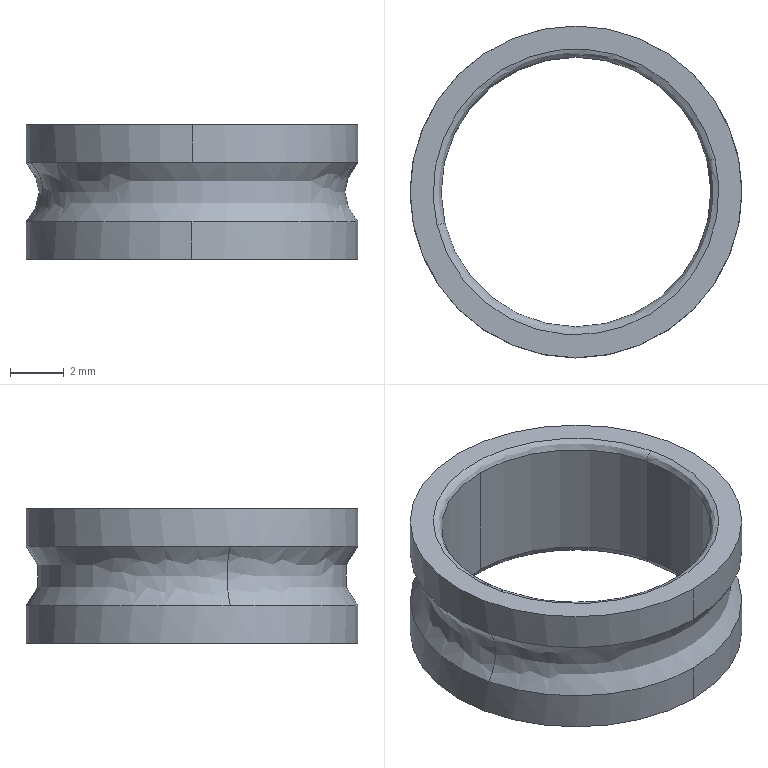Part | SolidWorks | features BaseBody 1 | 1 solid | 14 faces | box 12.3 x 12.3 x 5 mm | volume 173.294 mm3 | spline 6 | cylinder 6 | plane 2 | commonest cylinder face diameters 12.3 x4 10 x2
STEP:
#1=CARTESIAN_POINT('',(465.27,-93.215,300.844));
#2=VERTEX_POINT('',#1);
#3=CARTESIAN_POINT('',(460.405,-99.367,300.844));
#4=VERTEX_POINT('',#3);
#5=CARTESIAN_POINT('',(465.27,-98.215,300.844));
#6=DIRECTION('',(0.000000004,-0.00000001,1.));
#7=DIRECTION('',(0.,1.,0.00000001));
#8=AXIS2_PLACEMENT_3D('',#5,#6,#7);
#9=CIRCLE('',#8,5.);
#10=EDGE_CURVE('',#2,#4,#9,.T.);
#11=ORIENTED_EDGE('',*,*,#10,.T.);
#12=CARTESIAN_POINT('',(460.113,-99.436,300.544));
#13=VERTEX_POINT('',#12);
#14=CARTESIAN_POINT('',(460.113,-99.436,300.844));
#15=DIRECTION('',(-0.2304,0.9731,0.00000001));
#16=DIRECTION('',(-0.9731,-0.2304,0.000000002));
#17=AXIS2_PLACEMENT_3D('',#14,#15,#16);
#18=CIRCLE('',#17,0.3);
#19=EDGE_CURVE('',#4,#13,#18,.T.);
#20=ORIENTED_EDGE('',*,*,#19,.T.);
#21=CARTESIAN_POINT('',(470.428,-96.994,300.544));
#22=VERTEX_POINT('',#21);
#23=CARTESIAN_POINT('',(460.113,-99.436,300.544));
#24=CARTESIAN_POINT('',(457.671,-89.121,300.544));
#25=CARTESIAN_POINT('',(467.985,-86.679,300.544));
#26=CARTESIAN_POINT('',(470.428,-96.994,300.544));
#27=(BOUNDED_CURVE()B_SPLINE_CURVE(3,(#23,#24,#25,#26),.UNSPECIFIED.,.F.,.F.)B_SPLINE_CURVE_WITH_KNOTS((4,4),(0.,1.),.UNSPECIFIED.)CURVE()GEOMETRIC_REPRESENTATION_ITEM()RATIONAL_B_SPLINE_CURVE((1.,0.3333,0.3333,1.))REPRESENTATION_ITEM(''));
#28=EDGE_CURVE('',#13,#22,#27,.T.);
#29=ORIENTED_EDGE('',*,*,#28,.T.);
#30=CARTESIAN_POINT('',(470.136,-97.063,300.844));
#31=VERTEX_POINT('',#30);
#32=CARTESIAN_POINT('',(470.428,-96.994,300.844));
#33=DIRECTION('',(0.2304,-0.9731,-0.00000001));
#34=DIRECTION('',(0.9731,0.2304,-0.000000002));
#35=AXIS2_PLACEMENT_3D('',#32,#33,#34);
#36=CIRCLE('',#35,0.3);
#37=EDGE_CURVE('',#31,#22,#36,.T.);
#38=ORIENTED_EDGE('',*,*,#37,.F.);
#39=CARTESIAN_POINT('',(465.27,-98.215,300.844));
#40=DIRECTION('',(0.000000004,-0.00000001,1.));
#41=DIRECTION('',(0.,1.,0.00000001));
#42=AXIS2_PLACEMENT_3D('',#39,#40,#41);
#43=CIRCLE('',#42,5.);
#44=EDGE_CURVE('',#31,#2,#43,.T.);
#45=ORIENTED_EDGE('',*,*,#44,.T.);
#46=EDGE_LOOP('',(#11,#20,#29,#38,#45));
#47=FACE_OUTER_BOUND('',#46,.T.);
#48=CARTESIAN_POINT('',(460.405,-99.367,300.844));
#49=CARTESIAN_POINT('',(458.101,-89.636,300.844));
#50=CARTESIAN_POINT('',(467.832,-87.332,300.844));
#51=CARTESIAN_POINT('',(470.136,-97.063,300.844));
#52=CARTESIAN_POINT('',(460.405,-99.367,300.669));
#53=CARTESIAN_POINT('',(458.101,-89.636,300.669));
#54=CARTESIAN_POINT('',(467.832,-87.332,300.669));
#55=CARTESIAN_POINT('',(470.136,-97.063,300.669));
#56=CARTESIAN_POINT('',(460.284,-99.396,300.544));
#57=CARTESIAN_POINT('',(457.923,-89.423,300.544));
#58=CARTESIAN_POINT('',(467.895,-87.062,300.544));
#59=CARTESIAN_POINT('',(470.257,-97.034,300.544));
#60=CARTESIAN_POINT('',(460.113,-99.436,300.544));
#61=CARTESIAN_POINT('',(457.671,-89.121,300.544));
#62=CARTESIAN_POINT('',(467.985,-86.679,300.544));
#63=CARTESIAN_POINT('',(470.428,-96.994,300.544));
#64=(BOUNDED_SURFACE()B_SPLINE_SURFACE(3,3,((#48,#49,#50,#51),(#52,#53,#54,#55),(#56,#57,#58,#59),(#60,#61,#62,#63)),.UNSPECIFIED.,.F.,.F.,.T.)B_SPLINE_SURFACE_WITH_KNOTS((4,4),(4,4),(0.,1.),(0.,1.),.UNSPECIFIED.)GEOMETRIC_REPRESENTATION_ITEM()RATIONAL_B_SPLINE_SURFACE(((1.,0.3333,0.3333,1.),(0.8047,0.2682,0.2682,0.8047),(0.8047,0.2682,0.2682,0.8047),(1.,0.3333,0.3333,1.)))REPRESENTATION_ITEM('')SURFACE());
#65=ADVANCED_FACE('',(#47),#64,.T.);
#66=CARTESIAN_POINT('',(470.428,-96.994,305.544));
#67=VERTEX_POINT('',#66);
#68=CARTESIAN_POINT('',(460.113,-99.436,305.544));
#69=VERTEX_POINT('',#68);
#70=CARTESIAN_POINT('',(470.428,-96.994,305.544));
#71=CARTESIAN_POINT('',(467.985,-86.679,305.544));
#72=CARTESIAN_POINT('',(457.671,-89.121,305.544));
#73=CARTESIAN_POINT('',(460.113,-99.436,305.544));
#74=(BOUNDED_CURVE()B_SPLINE_CURVE(3,(#70,#71,#72,#73),.UNSPECIFIED.,.F.,.T.)B_SPLINE_CURVE_WITH_KNOTS((4,4),(0.,1.),.UNSPECIFIED.)CURVE()GEOMETRIC_REPRESENTATION_ITEM()RATIONAL_B_SPLINE_CURVE((1.,0.3333,0.3333,1.))REPRESENTATION_ITEM(''));
#75=EDGE_CURVE('',#67,#69,#74,.T.);
#76=ORIENTED_EDGE('',*,*,#75,.T.);
#77=CARTESIAN_POINT('',(460.405,-99.367,305.244));
#78=VERTEX_POINT('',#77);
#79=CARTESIAN_POINT('',(460.113,-99.436,305.244));
#80=DIRECTION('',(-0.2304,0.9731,0.00000001));
#81=DIRECTION('',(-0.9731,-0.2304,0.000000002));
#82=AXIS2_PLACEMENT_3D('',#79,#80,#81);
#83=CIRCLE('',#82,0.3);
#84=EDGE_CURVE('',#69,#78,#83,.T.);
#85=ORIENTED_EDGE('',*,*,#84,.T.);
#86=CARTESIAN_POINT('',(465.27,-93.215,305.244));
#87=VERTEX_POINT('',#86);
#88=CARTESIAN_POINT('',(465.27,-98.215,305.244));
#89=DIRECTION('',(-0.000000004,0.00000001,-1.));
#90=DIRECTION('',(0.,1.,0.00000001));
#91=AXIS2_PLACEMENT_3D('',#88,#89,#90);
#92=CIRCLE('',#91,5.);
#93=EDGE_CURVE('',#78,#87,#92,.T.);
#94=ORIENTED_EDGE('',*,*,#93,.T.);
#95=CARTESIAN_POINT('',(470.136,-97.063,305.244));
#96=VERTEX_POINT('',#95);
#97=CARTESIAN_POINT('',(465.27,-98.215,305.244));
#98=DIRECTION('',(-0.000000004,0.00000001,-1.));
#99=DIRECTION('',(0.,1.,0.00000001));
#100=AXIS2_PLACEMENT_3D('',#97,#98,#99);
#101=CIRCLE('',#100,5.);
#102=EDGE_CURVE('',#87,#96,#101,.T.);
#103=ORIENTED_EDGE('',*,*,#102,.T.);
#104=CARTESIAN_POINT('',(470.428,-96.994,305.244));
#105=DIRECTION('',(0.2304,-0.9731,-0.00000001));
#106=DIRECTION('',(0.9731,0.2304,-0.000000002));
#107=AXIS2_PLACEMENT_3D('',#104,#105,#106);
#108=CIRCLE('',#107,0.3);
#109=EDGE_CURVE('',#67,#96,#108,.T.);
#110=ORIENTED_EDGE('',*,*,#109,.F.);
#111=EDGE_LOOP('',(#76,#85,#94,#103,#110));
#112=FACE_OUTER_BOUND('',#111,.T.);
#113=CARTESIAN_POINT('',(460.113,-99.436,305.544));
#114=CARTESIAN_POINT('',(457.671,-89.121,305.544));
#115=CARTESIAN_POINT('',(467.985,-86.679,305.544));
#116=CARTESIAN_POINT('',(470.428,-96.994,305.544));
#117=CARTESIAN_POINT('',(460.284,-99.396,305.544));
#118=CARTESIAN_POINT('',(457.923,-89.423,305.544));
#119=CARTESIAN_POINT('',(467.895,-87.062,305.544));
#120=CARTESIAN_POINT('',(470.257,-97.034,305.544));
#121=CARTESIAN_POINT('',(460.405,-99.367,305.42));
#122=CARTESIAN_POINT('',(458.101,-89.636,305.42));
#123=CARTESIAN_POINT('',(467.832,-87.332,305.42));
#124=CARTESIAN_POINT('',(470.136,-97.063,305.42));
#125=CARTESIAN_POINT('',(460.405,-99.367,305.244));
#126=CARTESIAN_POINT('',(458.101,-89.636,305.244));
#127=CARTESIAN_POINT('',(467.832,-87.332,305.244));
#128=CARTESIAN_POINT('',(470.136,-97.063,305.244));
#129=(BOUNDED_SURFACE()B_SPLINE_SURFACE(3,3,((#113,#114,#115,#116),(#117,#118,#119,#120),(#121,#122,#123,#124),(#125,#126,#127,#128)),.UNSPECIFIED.,.F.,.F.,.T.)B_SPLINE_SURFACE_WITH_KNOTS((4,4),(4,4),(0.,1.),(0.,1.),.UNSPECIFIED.)GEOMETRIC_REPRESENTATION_ITEM()RATIONAL_B_SPLINE_SURFACE(((1.,0.3333,0.3333,1.),(0.8047,0.2682,0.2682,0.8047),(0.8047,0.2682,0.2682,0.8047),(1.,0.3333,0.3333,1.)))REPRESENTATION_ITEM('')SURFACE());
#130=ADVANCED_FACE('',(#112),#129,.T.);
#131=CARTESIAN_POINT('',(459.286,-99.632,304.139));
#132=VERTEX_POINT('',#131);
#133=CARTESIAN_POINT('',(465.27,-104.365,304.139));
#134=VERTEX_POINT('',#133);
#135=CARTESIAN_POINT('',(465.27,-98.215,304.139));
#136=DIRECTION('',(0.000000004,-0.00000001,1.));
#137=DIRECTION('',(0.,1.,0.00000001));
#138=AXIS2_PLACEMENT_3D('',#135,#136,#137);
#139=CIRCLE('',#138,6.15);
#140=EDGE_CURVE('',#132,#134,#139,.T.);
#141=ORIENTED_EDGE('',*,*,#140,.F.);
#142=CARTESIAN_POINT('',(459.286,-99.632,301.949));
#143=VERTEX_POINT('',#142);
#144=CARTESIAN_POINT('',(458.288,-99.868,303.044));
#145=DIRECTION('',(-0.2304,0.9731,0.00000001));
#146=DIRECTION('',(-0.9731,-0.2304,0.000000002));
#147=AXIS2_PLACEMENT_3D('',#144,#145,#146);
#148=CIRCLE('',#147,1.5);
#149=EDGE_CURVE('',#132,#143,#148,.T.);
#150=ORIENTED_EDGE('',*,*,#149,.T.);
#151=CARTESIAN_POINT('',(465.27,-104.365,301.949));
#152=VERTEX_POINT('',#151);
#153=CARTESIAN_POINT('',(465.27,-98.215,301.949));
#154=DIRECTION('',(-0.000000004,0.00000001,-1.));
#155=DIRECTION('',(0.,1.,0.00000001));
#156=AXIS2_PLACEMENT_3D('',#153,#154,#155);
#157=CIRCLE('',#156,6.15);
#158=EDGE_CURVE('',#152,#143,#157,.T.);
#159=ORIENTED_EDGE('',*,*,#158,.F.);
#160=CARTESIAN_POINT('',(471.255,-96.798,301.949));
#161=VERTEX_POINT('',#160);
#162=CARTESIAN_POINT('',(465.27,-98.215,301.949));
#163=DIRECTION('',(-0.000000004,0.00000001,-1.));
#164=DIRECTION('',(0.,1.,0.00000001));
#165=AXIS2_PLACEMENT_3D('',#162,#163,#164);
#166=CIRCLE('',#165,6.15);
#167=EDGE_CURVE('',#161,#152,#166,.T.);
#168=ORIENTED_EDGE('',*,*,#167,.F.);
#169=CARTESIAN_POINT('',(471.255,-96.798,304.139));
#170=VERTEX_POINT('',#169);
#171=CARTESIAN_POINT('',(472.252,-96.562,303.044));
#172=DIRECTION('',(0.2304,-0.9731,-0.00000001));
#173=DIRECTION('',(0.9731,0.2304,-0.000000002));
#174=AXIS2_PLACEMENT_3D('',#171,#172,#173);
#175=CIRCLE('',#174,1.5);
#176=EDGE_CURVE('',#170,#161,#175,.T.);
#177=ORIENTED_EDGE('',*,*,#176,.F.);
#178=CARTESIAN_POINT('',(465.27,-98.215,304.139));
#179=DIRECTION('',(0.000000004,-0.00000001,1.));
#180=DIRECTION('',(0.,1.,0.00000001));
#181=AXIS2_PLACEMENT_3D('',#178,#179,#180);
#182=CIRCLE('',#181,6.15);
#183=EDGE_CURVE('',#134,#170,#182,.T.);
#184=ORIENTED_EDGE('',*,*,#183,.F.);
#185=EDGE_LOOP('',(#141,#150,#159,#168,#177,#184));
#186=FACE_OUTER_BOUND('',#185,.T.);
#187=CARTESIAN_POINT('',(471.255,-96.798,304.139));
#188=CARTESIAN_POINT('',(474.089,-108.767,304.139));
#189=CARTESIAN_POINT('',(462.12,-111.601,304.139));
#190=CARTESIAN_POINT('',(459.286,-99.632,304.139));
#191=CARTESIAN_POINT('',(470.597,-96.954,303.507));
#192=CARTESIAN_POINT('',(473.12,-107.608,303.507));
#193=CARTESIAN_POINT('',(462.466,-110.13,303.507));
#194=CARTESIAN_POINT('',(459.943,-99.476,303.507));
#195=CARTESIAN_POINT('',(470.597,-96.954,302.582));
#196=CARTESIAN_POINT('',(473.12,-107.608,302.582));
#197=CARTESIAN_POINT('',(462.466,-110.13,302.582));
#198=CARTESIAN_POINT('',(459.943,-99.476,302.582));
#199=CARTESIAN_POINT('',(471.255,-96.798,301.949));
#200=CARTESIAN_POINT('',(474.089,-108.767,301.949));
#201=CARTESIAN_POINT('',(462.12,-111.601,301.949));
#202=CARTESIAN_POINT('',(459.286,-99.632,301.949));
#203=(BOUNDED_SURFACE()B_SPLINE_SURFACE(3,3,((#187,#188,#189,#190),(#191,#192,#193,#194),(#195,#196,#197,#198),(#199,#200,#201,#202)),.UNSPECIFIED.,.F.,.F.,.T.)B_SPLINE_SURFACE_WITH_KNOTS((4,4),(4,4),(0.,1.),(0.,1.),.UNSPECIFIED.)GEOMETRIC_REPRESENTATION_ITEM()RATIONAL_B_SPLINE_SURFACE(((1.,0.3333,0.3333,1.),(0.7889,0.263,0.263,0.7889),(0.7889,0.263,0.263,0.7889),(1.,0.3333,0.3333,1.)))REPRESENTATION_ITEM('')SURFACE());
#204=ADVANCED_FACE('',(#186),#203,.F.);
#205=CARTESIAN_POINT('',(465.27,-103.215,305.244));
#206=VERTEX_POINT('',#205);
#207=CARTESIAN_POINT('',(465.27,-98.215,305.244));
#208=DIRECTION('',(-0.000000004,0.00000001,-1.));
#209=DIRECTION('',(0.,1.,0.00000001));
#210=AXIS2_PLACEMENT_3D('',#207,#208,#209);
#211=CIRCLE('',#210,5.);
#212=EDGE_CURVE('',#206,#78,#211,.T.);
#213=ORIENTED_EDGE('',*,*,#212,.F.);
#214=CARTESIAN_POINT('',(465.27,-103.215,300.844));
#215=VERTEX_POINT('',#214);
#216=CARTESIAN_POINT('',(465.27,-103.215,303.044));
#217=DIRECTION('',(-0.000000004,0.00000001,-1.));
#218=VECTOR('',#217,1000.);
#219=LINE('',#216,#218);
#220=EDGE_CURVE('',#206,#215,#219,.T.);
#221=ORIENTED_EDGE('',*,*,#220,.T.);
#222=CARTESIAN_POINT('',(465.27,-98.215,300.844));
#223=DIRECTION('',(0.000000004,-0.00000001,1.));
#224=DIRECTION('',(0.,1.,0.00000001));
#225=AXIS2_PLACEMENT_3D('',#222,#223,#224);
#226=CIRCLE('',#225,5.);
#227=EDGE_CURVE('',#4,#215,#226,.T.);
#228=ORIENTED_EDGE('',*,*,#227,.F.);
#229=ORIENTED_EDGE('',*,*,#10,.F.);
#230=CARTESIAN_POINT('',(465.27,-93.215,303.044));
#231=DIRECTION('',(-0.000000004,0.00000001,-1.));
#232=VECTOR('',#231,1000.);
#233=LINE('',#230,#232);
#234=EDGE_CURVE('',#87,#2,#233,.T.);
#235=ORIENTED_EDGE('',*,*,#234,.F.);
#236=ORIENTED_EDGE('',*,*,#93,.F.);
#237=EDGE_LOOP('',(#213,#221,#228,#229,#235,#236));
#238=FACE_OUTER_BOUND('',#237,.T.);
#239=CARTESIAN_POINT('',(465.27,-98.215,303.044));
#240=DIRECTION('',(-0.000000004,0.00000001,-1.));
#241=DIRECTION('',(0.,1.,0.00000001));
#242=AXIS2_PLACEMENT_3D('',#239,#240,#241);
#243=CYLINDRICAL_SURFACE('',#242,5.);
#244=ADVANCED_FACE('',(#238),#243,.F.);
#245=CARTESIAN_POINT('',(465.27,-92.065,301.949));
#246=VERTEX_POINT('',#245);
#247=CARTESIAN_POINT('',(465.27,-98.215,301.949));
#248=DIRECTION('',(-0.000000004,0.00000001,-1.));
#249=DIRECTION('',(0.,1.,0.00000001));
#250=AXIS2_PLACEMENT_3D('',#247,#248,#249);
#251=CIRCLE('',#250,6.15);
#252=EDGE_CURVE('',#246,#161,#251,.T.);
#253=ORIENTED_EDGE('',*,*,#252,.T.);
#254=ORIENTED_EDGE('',*,*,#167,.T.);
#255=CARTESIAN_POINT('',(465.27,-104.365,300.544));
#256=VERTEX_POINT('',#255);
#257=CARTESIAN_POINT('',(465.27,-104.365,301.247));
#258=DIRECTION('',(-0.000000004,0.00000001,-1.));
#259=VECTOR('',#258,1000.);
#260=LINE('',#257,#259);
#261=EDGE_CURVE('',#152,#256,#260,.T.);
#262=ORIENTED_EDGE('',*,*,#261,.T.);
#263=CARTESIAN_POINT('',(465.27,-92.065,300.544));
#264=VERTEX_POINT('',#263);
#265=CARTESIAN_POINT('',(465.27,-98.215,300.544));
#266=DIRECTION('',(-0.000000004,0.00000001,-1.));
#267=DIRECTION('',(0.,1.,0.00000001));
#268=AXIS2_PLACEMENT_3D('',#265,#266,#267);
#269=CIRCLE('',#268,6.15);
#270=EDGE_CURVE('',#264,#256,#269,.T.);
#271=ORIENTED_EDGE('',*,*,#270,.F.);
#272=CARTESIAN_POINT('',(465.27,-92.065,301.247));
#273=DIRECTION('',(-0.000000004,0.00000001,-1.));
#274=VECTOR('',#273,1000.);
#275=LINE('',#272,#274);
#276=EDGE_CURVE('',#246,#264,#275,.T.);
#277=ORIENTED_EDGE('',*,*,#276,.F.);
#278=EDGE_LOOP('',(#253,#254,#262,#271,#277));
#279=FACE_OUTER_BOUND('',#278,.T.);
#280=CARTESIAN_POINT('',(465.27,-98.215,301.247));
#281=DIRECTION('',(-0.000000004,0.00000001,-1.));
#282=DIRECTION('',(0.,1.,0.00000001));
#283=AXIS2_PLACEMENT_3D('',#280,#281,#282);
#284=CYLINDRICAL_SURFACE('',#283,6.15);
#285=ADVANCED_FACE('',(#279),#284,.T.);
#286=CARTESIAN_POINT('',(465.27,-104.365,305.544));
#287=VERTEX_POINT('',#286);
#288=CARTESIAN_POINT('',(465.27,-92.065,305.544));
#289=VERTEX_POINT('',#288);
#290=CARTESIAN_POINT('',(465.27,-98.215,305.544));
#291=DIRECTION('',(0.000000004,-0.00000001,1.));
#292=DIRECTION('',(0.,1.,0.00000001));
#293=AXIS2_PLACEMENT_3D('',#290,#291,#292);
#294=CIRCLE('',#293,6.15);
#295=EDGE_CURVE('',#287,#289,#294,.T.);
#296=ORIENTED_EDGE('',*,*,#295,.F.);
#297=CARTESIAN_POINT('',(465.27,-104.365,304.842));
#298=DIRECTION('',(-0.000000004,0.00000001,-1.));
#299=VECTOR('',#298,1000.);
#300=LINE('',#297,#299);
#301=EDGE_CURVE('',#287,#134,#300,.T.);
#302=ORIENTED_EDGE('',*,*,#301,.T.);
#303=ORIENTED_EDGE('',*,*,#183,.T.);
#304=CARTESIAN_POINT('',(465.27,-92.065,304.139));
#305=VERTEX_POINT('',#304);
#306=CARTESIAN_POINT('',(465.27,-98.215,304.139));
#307=DIRECTION('',(0.000000004,-0.00000001,1.));
#308=DIRECTION('',(0.,1.,0.00000001));
#309=AXIS2_PLACEMENT_3D('',#306,#307,#308);
#310=CIRCLE('',#309,6.15);
#311=EDGE_CURVE('',#170,#305,#310,.T.);
#312=ORIENTED_EDGE('',*,*,#311,.T.);
#313=CARTESIAN_POINT('',(465.27,-92.065,304.842));
#314=DIRECTION('',(-0.000000004,0.00000001,-1.));
#315=VECTOR('',#314,1000.);
#316=LINE('',#313,#315);
#317=EDGE_CURVE('',#289,#305,#316,.T.);
#318=ORIENTED_EDGE('',*,*,#317,.F.);
#319=EDGE_LOOP('',(#296,#302,#303,#312,#318));
#320=FACE_OUTER_BOUND('',#319,.T.);
#321=CARTESIAN_POINT('',(465.27,-98.215,304.842));
#322=DIRECTION('',(-0.000000004,0.00000001,-1.));
#323=DIRECTION('',(0.,1.,0.00000001));
#324=AXIS2_PLACEMENT_3D('',#321,#322,#323);
#325=CYLINDRICAL_SURFACE('',#324,6.15);
#326=ADVANCED_FACE('',(#320),#325,.T.);
#327=ORIENTED_EDGE('',*,*,#220,.F.);
#328=CARTESIAN_POINT('',(465.27,-98.215,305.244));
#329=DIRECTION('',(-0.000000004,0.00000001,-1.));
#330=DIRECTION('',(0.,1.,0.00000001));
#331=AXIS2_PLACEMENT_3D('',#328,#329,#330);
#332=CIRCLE('',#331,5.);
#333=EDGE_CURVE('',#96,#206,#332,.T.);
#334=ORIENTED_EDGE('',*,*,#333,.F.);
#335=ORIENTED_EDGE('',*,*,#102,.F.);
#336=ORIENTED_EDGE('',*,*,#234,.T.);
#337=ORIENTED_EDGE('',*,*,#44,.F.);
#338=CARTESIAN_POINT('',(465.27,-98.215,300.844));
#339=DIRECTION('',(0.000000004,-0.00000001,1.));
#340=DIRECTION('',(0.,1.,0.00000001));
#341=AXIS2_PLACEMENT_3D('',#338,#339,#340);
#342=CIRCLE('',#341,5.);
#343=EDGE_CURVE('',#215,#31,#342,.T.);
#344=ORIENTED_EDGE('',*,*,#343,.F.);
#345=EDGE_LOOP('',(#327,#334,#335,#336,#337,#344));
#346=FACE_OUTER_BOUND('',#345,.T.);
#347=CARTESIAN_POINT('',(465.27,-98.215,303.044));
#348=DIRECTION('',(-0.000000004,0.00000001,-1.));
#349=DIRECTION('',(0.,1.,0.00000001));
#350=AXIS2_PLACEMENT_3D('',#347,#348,#349);
#351=CYLINDRICAL_SURFACE('',#350,5.);
#352=ADVANCED_FACE('',(#346),#351,.F.);
#353=ORIENTED_EDGE('',*,*,#19,.F.);
#354=ORIENTED_EDGE('',*,*,#227,.T.);
#355=ORIENTED_EDGE('',*,*,#343,.T.);
#356=ORIENTED_EDGE('',*,*,#37,.T.);
#357=CARTESIAN_POINT('',(470.428,-96.994,300.544));
#358=CARTESIAN_POINT('',(472.87,-107.309,300.544));
#359=CARTESIAN_POINT('',(462.555,-109.751,300.544));
#360=CARTESIAN_POINT('',(460.113,-99.436,300.544));
#361=(BOUNDED_CURVE()B_SPLINE_CURVE(3,(#357,#358,#359,#360),.UNSPECIFIED.,.F.,.T.)B_SPLINE_CURVE_WITH_KNOTS((4,4),(0.,1.),.UNSPECIFIED.)CURVE()GEOMETRIC_REPRESENTATION_ITEM()RATIONAL_B_SPLINE_CURVE((1.,0.3333,0.3333,1.))REPRESENTATION_ITEM(''));
#362=EDGE_CURVE('',#22,#13,#361,.T.);
#363=ORIENTED_EDGE('',*,*,#362,.T.);
#364=EDGE_LOOP('',(#353,#354,#355,#356,#363));
#365=FACE_OUTER_BOUND('',#364,.T.);
#366=CARTESIAN_POINT('',(470.136,-97.063,300.844));
#367=CARTESIAN_POINT('',(472.44,-106.794,300.844));
#368=CARTESIAN_POINT('',(462.709,-109.098,300.844));
#369=CARTESIAN_POINT('',(460.405,-99.367,300.844));
#370=CARTESIAN_POINT('',(470.136,-97.063,300.669));
#371=CARTESIAN_POINT('',(472.44,-106.794,300.669));
#372=CARTESIAN_POINT('',(462.709,-109.098,300.669));
#373=CARTESIAN_POINT('',(460.405,-99.367,300.669));
#374=CARTESIAN_POINT('',(470.257,-97.034,300.544));
#375=CARTESIAN_POINT('',(472.618,-107.007,300.544));
#376=CARTESIAN_POINT('',(462.645,-109.368,300.544));
#377=CARTESIAN_POINT('',(460.284,-99.396,300.544));
#378=CARTESIAN_POINT('',(470.428,-96.994,300.544));
#379=CARTESIAN_POINT('',(472.87,-107.309,300.544));
#380=CARTESIAN_POINT('',(462.555,-109.751,300.544));
#381=CARTESIAN_POINT('',(460.113,-99.436,300.544));
#382=(BOUNDED_SURFACE()B_SPLINE_SURFACE(3,3,((#366,#367,#368,#369),(#370,#371,#372,#373),(#374,#375,#376,#377),(#378,#379,#380,#381)),.UNSPECIFIED.,.F.,.F.,.T.)B_SPLINE_SURFACE_WITH_KNOTS((4,4),(4,4),(0.,1.),(0.,1.),.UNSPECIFIED.)GEOMETRIC_REPRESENTATION_ITEM()RATIONAL_B_SPLINE_SURFACE(((1.,0.3333,0.3333,1.),(0.8047,0.2682,0.2682,0.8047),(0.8047,0.2682,0.2682,0.8047),(1.,0.3333,0.3333,1.)))REPRESENTATION_ITEM('')SURFACE());
#383=ADVANCED_FACE('',(#365),#382,.T.);
#384=ORIENTED_EDGE('',*,*,#84,.F.);
#385=CARTESIAN_POINT('',(460.113,-99.436,305.544));
#386=CARTESIAN_POINT('',(462.555,-109.751,305.544));
#387=CARTESIAN_POINT('',(472.87,-107.309,305.544));
#388=CARTESIAN_POINT('',(470.428,-96.994,305.544));
#389=(BOUNDED_CURVE()B_SPLINE_CURVE(3,(#385,#386,#387,#388),.UNSPECIFIED.,.F.,.T.)B_SPLINE_CURVE_WITH_KNOTS((4,4),(0.,1.),.UNSPECIFIED.)CURVE()GEOMETRIC_REPRESENTATION_ITEM()RATIONAL_B_SPLINE_CURVE((1.,0.3333,0.3333,1.))REPRESENTATION_ITEM(''));
#390=EDGE_CURVE('',#69,#67,#389,.T.);
#391=ORIENTED_EDGE('',*,*,#390,.T.);
#392=ORIENTED_EDGE('',*,*,#109,.T.);
#393=ORIENTED_EDGE('',*,*,#333,.T.);
#394=ORIENTED_EDGE('',*,*,#212,.T.);
#395=EDGE_LOOP('',(#384,#391,#392,#393,#394));
#396=FACE_OUTER_BOUND('',#395,.T.);
#397=CARTESIAN_POINT('',(470.428,-96.994,305.544));
#398=CARTESIAN_POINT('',(472.87,-107.309,305.544));
#399=CARTESIAN_POINT('',(462.555,-109.751,305.544));
#400=CARTESIAN_POINT('',(460.113,-99.436,305.544));
#401=CARTESIAN_POINT('',(470.257,-97.034,305.544));
#402=CARTESIAN_POINT('',(472.618,-107.007,305.544));
#403=CARTESIAN_POINT('',(462.645,-109.368,305.544));
#404=CARTESIAN_POINT('',(460.284,-99.396,305.544));
#405=CARTESIAN_POINT('',(470.136,-97.063,305.42));
#406=CARTESIAN_POINT('',(472.44,-106.794,305.42));
#407=CARTESIAN_POINT('',(462.709,-109.098,305.42));
#408=CARTESIAN_POINT('',(460.405,-99.367,305.42));
#409=CARTESIAN_POINT('',(470.136,-97.063,305.244));
#410=CARTESIAN_POINT('',(472.44,-106.794,305.244));
#411=CARTESIAN_POINT('',(462.709,-109.098,305.244));
#412=CARTESIAN_POINT('',(460.405,-99.367,305.244));
#413=(BOUNDED_SURFACE()B_SPLINE_SURFACE(3,3,((#397,#398,#399,#400),(#401,#402,#403,#404),(#405,#406,#407,#408),(#409,#410,#411,#412)),.UNSPECIFIED.,.F.,.F.,.T.)B_SPLINE_SURFACE_WITH_KNOTS((4,4),(4,4),(0.,1.),(0.,1.),.UNSPECIFIED.)GEOMETRIC_REPRESENTATION_ITEM()RATIONAL_B_SPLINE_SURFACE(((1.,0.3333,0.3333,1.),(0.8047,0.2682,0.2682,0.8047),(0.8047,0.2682,0.2682,0.8047),(1.,0.3333,0.3333,1.)))REPRESENTATION_ITEM('')SURFACE());
#414=ADVANCED_FACE('',(#396),#413,.T.);
#415=ORIENTED_EDGE('',*,*,#28,.F.);
#416=ORIENTED_EDGE('',*,*,#362,.F.);
#417=EDGE_LOOP('',(#415,#416));
#418=FACE_BOUND('',#417,.T.);
#419=ORIENTED_EDGE('',*,*,#270,.T.);
#420=CARTESIAN_POINT('',(465.27,-98.215,300.544));
#421=DIRECTION('',(-0.000000004,0.00000001,-1.));
#422=DIRECTION('',(0.,1.,0.00000001));
#423=AXIS2_PLACEMENT_3D('',#420,#421,#422);
#424=CIRCLE('',#423,6.15);
#425=EDGE_CURVE('',#256,#264,#424,.T.);
#426=ORIENTED_EDGE('',*,*,#425,.T.);
#427=EDGE_LOOP('',(#419,#426));
#428=FACE_OUTER_BOUND('',#427,.T.);
#429=CARTESIAN_POINT('',(470.841,-96.896,300.544));
#430=DIRECTION('',(-0.000000004,0.00000001,-1.));
#431=DIRECTION('',(0.,1.,0.00000001));
#432=AXIS2_PLACEMENT_3D('',#429,#430,#431);
#433=PLANE('',#432);
#434=ADVANCED_FACE('',(#418,#428),#433,.T.);
#435=CARTESIAN_POINT('',(465.27,-98.215,305.544));
#436=DIRECTION('',(0.000000004,-0.00000001,1.));
#437=DIRECTION('',(0.,1.,0.00000001));
#438=AXIS2_PLACEMENT_3D('',#435,#436,#437);
#439=CIRCLE('',#438,6.15);
#440=EDGE_CURVE('',#289,#287,#439,.T.);
#441=ORIENTED_EDGE('',*,*,#440,.T.);
#442=ORIENTED_EDGE('',*,*,#295,.T.);
#443=EDGE_LOOP('',(#441,#442));
#444=FACE_OUTER_BOUND('',#443,.T.);
#445=ORIENTED_EDGE('',*,*,#75,.F.);
#446=ORIENTED_EDGE('',*,*,#390,.F.);
#447=EDGE_LOOP('',(#445,#446));
#448=FACE_BOUND('',#447,.T.);
#449=CARTESIAN_POINT('',(470.841,-96.896,305.544));
#450=DIRECTION('',(0.000000004,-0.00000001,1.));
#451=DIRECTION('',(0.,-1.,-0.00000001));
#452=AXIS2_PLACEMENT_3D('',#449,#450,#451);
#453=PLANE('',#452);
#454=ADVANCED_FACE('',(#444,#448),#453,.T.);
#455=ORIENTED_EDGE('',*,*,#261,.F.);
#456=ORIENTED_EDGE('',*,*,#158,.T.);
#457=CARTESIAN_POINT('',(465.27,-98.215,301.949));
#458=DIRECTION('',(-0.000000004,0.00000001,-1.));
#459=DIRECTION('',(0.,1.,0.00000001));
#460=AXIS2_PLACEMENT_3D('',#457,#458,#459);
#461=CIRCLE('',#460,6.15);
#462=EDGE_CURVE('',#143,#246,#461,.T.);
#463=ORIENTED_EDGE('',*,*,#462,.T.);
#464=ORIENTED_EDGE('',*,*,#276,.T.);
#465=ORIENTED_EDGE('',*,*,#425,.F.);
#466=EDGE_LOOP('',(#455,#456,#463,#464,#465));
#467=FACE_OUTER_BOUND('',#466,.T.);
#468=CARTESIAN_POINT('',(465.27,-98.215,301.247));
#469=DIRECTION('',(-0.000000004,0.00000001,-1.));
#470=DIRECTION('',(0.,1.,0.00000001));
#471=AXIS2_PLACEMENT_3D('',#468,#469,#470);
#472=CYLINDRICAL_SURFACE('',#471,6.15);
#473=ADVANCED_FACE('',(#467),#472,.T.);
#474=ORIENTED_EDGE('',*,*,#301,.F.);
#475=ORIENTED_EDGE('',*,*,#440,.F.);
#476=ORIENTED_EDGE('',*,*,#317,.T.);
#477=CARTESIAN_POINT('',(465.27,-98.215,304.139));
#478=DIRECTION('',(0.000000004,-0.00000001,1.));
#479=DIRECTION('',(0.,1.,0.00000001));
#480=AXIS2_PLACEMENT_3D('',#477,#478,#479);
#481=CIRCLE('',#480,6.15);
#482=EDGE_CURVE('',#305,#132,#481,.T.);
#483=ORIENTED_EDGE('',*,*,#482,.T.);
#484=ORIENTED_EDGE('',*,*,#140,.T.);
#485=EDGE_LOOP('',(#474,#475,#476,#483,#484));
#486=FACE_OUTER_BOUND('',#485,.T.);
#487=CARTESIAN_POINT('',(465.27,-98.215,304.842));
#488=DIRECTION('',(-0.000000004,0.00000001,-1.));
#489=DIRECTION('',(0.,1.,0.00000001));
#490=AXIS2_PLACEMENT_3D('',#487,#488,#489);
#491=CYLINDRICAL_SURFACE('',#490,6.15);
#492=ADVANCED_FACE('',(#486),#491,.T.);
#493=ORIENTED_EDGE('',*,*,#149,.F.);
#494=ORIENTED_EDGE('',*,*,#482,.F.);
#495=ORIENTED_EDGE('',*,*,#311,.F.);
#496=ORIENTED_EDGE('',*,*,#176,.T.);
#497=ORIENTED_EDGE('',*,*,#252,.F.);
#498=ORIENTED_EDGE('',*,*,#462,.F.);
#499=EDGE_LOOP('',(#493,#494,#495,#496,#497,#498));
#500=FACE_OUTER_BOUND('',#499,.T.);
#501=CARTESIAN_POINT('',(459.286,-99.632,304.139));
#502=CARTESIAN_POINT('',(456.452,-87.663,304.139));
#503=CARTESIAN_POINT('',(468.421,-84.829,304.139));
#504=CARTESIAN_POINT('',(471.255,-96.798,304.139));
#505=CARTESIAN_POINT('',(459.943,-99.476,303.507));
#506=CARTESIAN_POINT('',(457.421,-88.822,303.507));
#507=CARTESIAN_POINT('',(468.075,-86.3,303.507));
#508=CARTESIAN_POINT('',(470.597,-96.954,303.507));
#509=CARTESIAN_POINT('',(459.943,-99.476,302.582));
#510=CARTESIAN_POINT('',(457.421,-88.822,302.582));
#511=CARTESIAN_POINT('',(468.075,-86.3,302.582));
#512=CARTESIAN_POINT('',(470.597,-96.954,302.582));
#513=CARTESIAN_POINT('',(459.286,-99.632,301.949));
#514=CARTESIAN_POINT('',(456.452,-87.663,301.949));
#515=CARTESIAN_POINT('',(468.421,-84.829,301.949));
#516=CARTESIAN_POINT('',(471.255,-96.798,301.949));
#517=(BOUNDED_SURFACE()B_SPLINE_SURFACE(3,3,((#501,#502,#503,#504),(#505,#506,#507,#508),(#509,#510,#511,#512),(#513,#514,#515,#516)),.UNSPECIFIED.,.F.,.F.,.F.)B_SPLINE_SURFACE_WITH_KNOTS((4,4),(4,4),(0.,1.),(0.,1.),.UNSPECIFIED.)GEOMETRIC_REPRESENTATION_ITEM()RATIONAL_B_SPLINE_SURFACE(((1.,0.3333,0.3333,1.),(0.7889,0.263,0.263,0.7889),(0.7889,0.263,0.263,0.7889),(1.,0.3333,0.3333,1.)))REPRESENTATION_ITEM('')SURFACE());
#518=ADVANCED_FACE('',(#500),#517,.F.);
#519=CLOSED_SHELL('',(#65,#130,#204,#244,#285,#326,#352,#383,#414,#434,#454,#473,#492,#518));
#520=MANIFOLD_SOLID_BREP('',#519);
#521=CARTESIAN_POINT('',(0.,0.,0.));
#522=DIRECTION('',(0.,0.,1.));
#523=DIRECTION('',(1.,0.,0.));
#524=AXIS2_PLACEMENT_3D('',#521,#522,#523);
#525=(LENGTH_UNIT()NAMED_UNIT(*)SI_UNIT(.MILLI.,.METRE.));
#526=UNCERTAINTY_MEASURE_WITH_UNIT(LENGTH_MEASURE(0.00001),#525,'','');
#527=(NAMED_UNIT(*)PLANE_ANGLE_UNIT()SI_UNIT($,.RADIAN.));
#528=(NAMED_UNIT(*)SI_UNIT($,.STERADIAN.)SOLID_ANGLE_UNIT());
#529=(GEOMETRIC_REPRESENTATION_CONTEXT(3)GLOBAL_UNCERTAINTY_ASSIGNED_CONTEXT((#526))GLOBAL_UNIT_ASSIGNED_CONTEXT((#525,#527,#528))REPRESENTATION_CONTEXT('',''));
#530=ADVANCED_BREP_SHAPE_REPRESENTATION('',(#520,#524),#529);